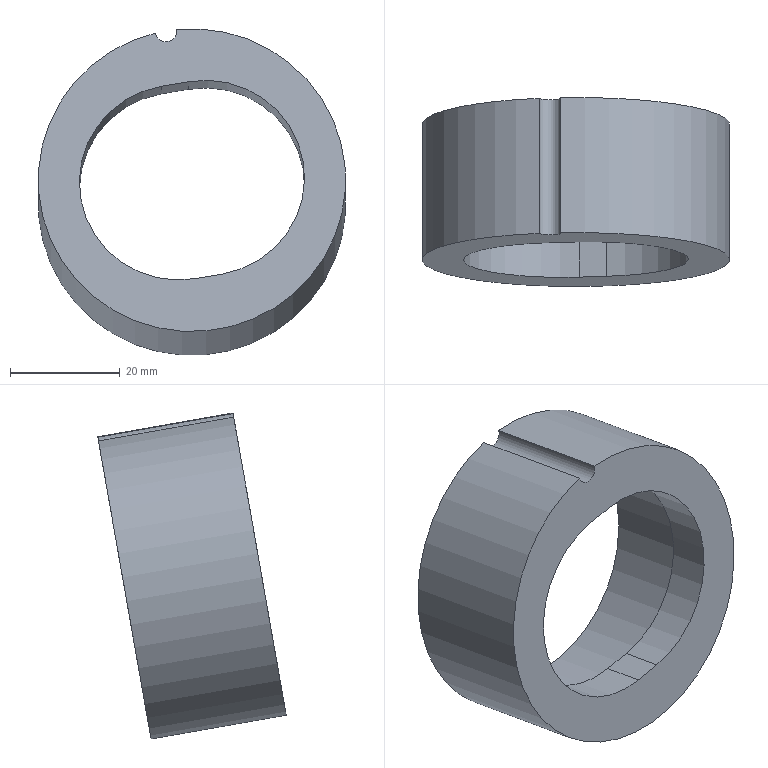Part | NX | features solid 2 | 1 solid | 10 faces | box 56 x 34.344 x 59.49 mm | volume 23536 mm3 | cylinder 5 | plane 5 | commonest cylinder face diameters 36.1 x2 4 x1 46 x1 56 x1
STEP:
#1=CARTESIAN_POINT('',(-417.763,-478.434,29.473));
#2=VERTEX_POINT('',#1);
#3=CARTESIAN_POINT('',(-417.763,-503.054,33.814));
#4=VERTEX_POINT('',#3);
#5=CARTESIAN_POINT('',(-417.763,-490.744,31.644));
#6=DIRECTION('',(0.,-0.9848,0.1736));
#7=VECTOR('',#6,1000.);
#8=LINE('',#5,#7);
#9=EDGE_CURVE('',#2,#4,#8,.T.);
#10=ORIENTED_EDGE('',*,*,#9,.T.);
#11=CARTESIAN_POINT('',(-421.702,-503.171,33.148));
#12=VERTEX_POINT('',#11);
#13=CARTESIAN_POINT('',(-415.006,-507.892,6.373));
#14=DIRECTION('',(0.,0.9848,-0.1736));
#15=DIRECTION('',(-0.1692,0.1711,0.9706));
#16=AXIS2_PLACEMENT_3D('',#13,#14,#15);
#17=CIRCLE('',#16,28.);
#18=EDGE_CURVE('',#4,#12,#17,.T.);
#19=ORIENTED_EDGE('',*,*,#18,.T.);
#20=CARTESIAN_POINT('',(-421.702,-478.551,28.807));
#21=VERTEX_POINT('',#20);
#22=CARTESIAN_POINT('',(-421.702,-490.861,30.977));
#23=DIRECTION('',(0.,-0.9848,0.1736));
#24=VECTOR('',#23,1000.);
#25=LINE('',#22,#24);
#26=EDGE_CURVE('',#12,#21,#25,.F.);
#27=ORIENTED_EDGE('',*,*,#26,.T.);
#28=CARTESIAN_POINT('',(-415.006,-483.272,2.032));
#29=DIRECTION('',(0.,0.9848,-0.1736));
#30=DIRECTION('',(-0.1692,0.1711,0.9706));
#31=AXIS2_PLACEMENT_3D('',#28,#29,#30);
#32=CIRCLE('',#31,28.);
#33=EDGE_CURVE('',#2,#21,#32,.T.);
#34=ORIENTED_EDGE('',*,*,#33,.F.);
#35=EDGE_LOOP('',(#10,#19,#27,#34));
#36=FACE_BOUND('',#35,.T.);
#37=CARTESIAN_POINT('',(-415.006,-483.272,2.032));
#38=DIRECTION('',(0.,-0.9848,0.1736));
#39=DIRECTION('',(-0.1692,0.1711,0.9706));
#40=AXIS2_PLACEMENT_3D('',#37,#38,#39);
#41=CYLINDRICAL_SURFACE('',#40,28.);
#42=ADVANCED_FACE('',(#36),#41,.T.);
#43=CARTESIAN_POINT('',(-418.898,-479.336,24.356));
#44=VERTEX_POINT('',#43);
#45=CARTESIAN_POINT('',(-415.006,-483.272,2.032));
#46=DIRECTION('',(0.,0.9848,-0.1736));
#47=DIRECTION('',(-0.1692,0.1711,0.9706));
#48=AXIS2_PLACEMENT_3D('',#45,#46,#47);
#49=CIRCLE('',#48,23.);
#50=EDGE_CURVE('',#44,#44,#49,.T.);
#51=ORIENTED_EDGE('',*,*,#50,.F.);
#52=EDGE_LOOP('',(#51));
#53=FACE_BOUND('',#52,.T.);
#54=ORIENTED_EDGE('',*,*,#33,.T.);
#55=CARTESIAN_POINT('',(-419.745,-478.48,29.209));
#56=DIRECTION('',(0.,0.9848,-0.1736));
#57=DIRECTION('',(-0.1692,0.1711,0.9706));
#58=AXIS2_PLACEMENT_3D('',#55,#56,#57);
#59=CIRCLE('',#58,2.);
#60=EDGE_CURVE('',#2,#21,#59,.T.);
#61=ORIENTED_EDGE('',*,*,#60,.F.);
#62=EDGE_LOOP('',(#54,#61));
#63=FACE_BOUND('',#62,.T.);
#64=CARTESIAN_POINT('',(-415.006,-483.272,2.032));
#65=DIRECTION('',(0.,-0.9848,0.1736));
#66=DIRECTION('',(-0.1692,0.1711,0.9706));
#67=AXIS2_PLACEMENT_3D('',#64,#65,#66);
#68=PLANE('',#67);
#69=ADVANCED_FACE('',(#53,#63),#68,.F.);
#70=CARTESIAN_POINT('',(-409.488,-510.908,-10.729));
#71=VERTEX_POINT('',#70);
#72=CARTESIAN_POINT('',(-414.415,-511.055,-11.563));
#73=VERTEX_POINT('',#72);
#74=CARTESIAN_POINT('',(-409.488,-510.908,-10.729));
#75=DIRECTION('',(-0.9856,-0.02939,-0.1667));
#76=VECTOR('',#75,1000.);
#77=LINE('',#74,#76);
#78=EDGE_CURVE('',#71,#73,#77,.T.);
#79=ORIENTED_EDGE('',*,*,#78,.T.);
#80=CARTESIAN_POINT('',(-420.525,-504.877,23.476));
#81=VERTEX_POINT('',#80);
#82=CARTESIAN_POINT('',(-417.47,-507.966,5.957));
#83=DIRECTION('',(0.,0.9848,-0.1736));
#84=DIRECTION('',(-0.1692,0.1711,0.9706));
#85=AXIS2_PLACEMENT_3D('',#82,#83,#84);
#86=CIRCLE('',#85,18.05);
#87=EDGE_CURVE('',#73,#81,#86,.T.);
#88=ORIENTED_EDGE('',*,*,#87,.T.);
#89=CARTESIAN_POINT('',(-415.597,-504.73,24.31));
#90=VERTEX_POINT('',#89);
#91=CARTESIAN_POINT('',(-415.597,-504.73,24.31));
#92=DIRECTION('',(-0.9856,-0.02939,-0.1667));
#93=VECTOR('',#92,1000.);
#94=LINE('',#91,#93);
#95=EDGE_CURVE('',#90,#81,#94,.T.);
#96=ORIENTED_EDGE('',*,*,#95,.F.);
#97=CARTESIAN_POINT('',(-412.542,-507.819,6.79));
#98=DIRECTION('',(0.,0.9848,-0.1736));
#99=DIRECTION('',(-0.1692,0.1711,0.9706));
#100=AXIS2_PLACEMENT_3D('',#97,#98,#99);
#101=CIRCLE('',#100,18.05);
#102=EDGE_CURVE('',#90,#71,#101,.T.);
#103=ORIENTED_EDGE('',*,*,#102,.T.);
#104=EDGE_LOOP('',(#79,#88,#96,#103));
#105=FACE_BOUND('',#104,.T.);
#106=CARTESIAN_POINT('',(-419.745,-503.1,33.55));
#107=DIRECTION('',(0.,0.9848,-0.1736));
#108=DIRECTION('',(-0.1692,0.1711,0.9706));
#109=AXIS2_PLACEMENT_3D('',#106,#107,#108);
#110=CIRCLE('',#109,2.);
#111=EDGE_CURVE('',#4,#12,#110,.T.);
#112=ORIENTED_EDGE('',*,*,#111,.T.);
#113=ORIENTED_EDGE('',*,*,#18,.F.);
#114=EDGE_LOOP('',(#112,#113));
#115=FACE_BOUND('',#114,.T.);
#116=CARTESIAN_POINT('',(-415.006,-507.892,6.373));
#117=DIRECTION('',(0.,-0.9848,0.1736));
#118=DIRECTION('',(-0.1692,0.1711,0.9706));
#119=AXIS2_PLACEMENT_3D('',#116,#117,#118);
#120=PLANE('',#119);
#121=ADVANCED_FACE('',(#105,#115),#120,.T.);
#122=ORIENTED_EDGE('',*,*,#50,.T.);
#123=EDGE_LOOP('',(#122));
#124=FACE_BOUND('',#123,.T.);
#125=CARTESIAN_POINT('',(-418.898,-496.078,27.308));
#126=VERTEX_POINT('',#125);
#127=CARTESIAN_POINT('',(-415.006,-500.014,4.984));
#128=DIRECTION('',(0.,0.9848,-0.1736));
#129=DIRECTION('',(-0.1692,0.1711,0.9706));
#130=AXIS2_PLACEMENT_3D('',#127,#128,#129);
#131=CIRCLE('',#130,23.);
#132=EDGE_CURVE('',#126,#126,#131,.T.);
#133=ORIENTED_EDGE('',*,*,#132,.F.);
#134=EDGE_LOOP('',(#133));
#135=FACE_BOUND('',#134,.T.);
#136=CARTESIAN_POINT('',(-415.006,-483.272,2.032));
#137=DIRECTION('',(0.,-0.9848,0.1736));
#138=DIRECTION('',(-0.1692,0.1711,0.9706));
#139=AXIS2_PLACEMENT_3D('',#136,#137,#138);
#140=CYLINDRICAL_SURFACE('',#139,23.);
#141=ADVANCED_FACE('',(#124,#135),#140,.F.);
#142=CARTESIAN_POINT('',(-415.597,-496.851,22.92));
#143=VERTEX_POINT('',#142);
#144=CARTESIAN_POINT('',(-409.488,-503.03,-12.118));
#145=VERTEX_POINT('',#144);
#146=CARTESIAN_POINT('',(-412.542,-499.941,5.401));
#147=DIRECTION('',(0.,0.9848,-0.1736));
#148=DIRECTION('',(-0.1692,0.1711,0.9706));
#149=AXIS2_PLACEMENT_3D('',#146,#147,#148);
#150=CIRCLE('',#149,18.05);
#151=EDGE_CURVE('',#143,#145,#150,.T.);
#152=ORIENTED_EDGE('',*,*,#151,.F.);
#153=CARTESIAN_POINT('',(-420.525,-496.998,22.087));
#154=VERTEX_POINT('',#153);
#155=CARTESIAN_POINT('',(-418.061,-496.925,22.504));
#156=DIRECTION('',(-0.9856,-0.02939,-0.1667));
#157=VECTOR('',#156,1000.);
#158=LINE('',#155,#157);
#159=EDGE_CURVE('',#143,#154,#158,.T.);
#160=ORIENTED_EDGE('',*,*,#159,.T.);
#161=CARTESIAN_POINT('',(-414.415,-503.177,-12.952));
#162=VERTEX_POINT('',#161);
#163=CARTESIAN_POINT('',(-417.47,-500.087,4.568));
#164=DIRECTION('',(0.,0.9848,-0.1736));
#165=DIRECTION('',(-0.1692,0.1711,0.9706));
#166=AXIS2_PLACEMENT_3D('',#163,#164,#165);
#167=CIRCLE('',#166,18.05);
#168=EDGE_CURVE('',#162,#154,#167,.T.);
#169=ORIENTED_EDGE('',*,*,#168,.F.);
#170=CARTESIAN_POINT('',(-411.952,-503.103,-12.535));
#171=DIRECTION('',(-0.9856,-0.02939,-0.1667));
#172=VECTOR('',#171,1000.);
#173=LINE('',#170,#172);
#174=EDGE_CURVE('',#145,#162,#173,.T.);
#175=ORIENTED_EDGE('',*,*,#174,.F.);
#176=EDGE_LOOP('',(#152,#160,#169,#175));
#177=FACE_BOUND('',#176,.T.);
#178=ORIENTED_EDGE('',*,*,#132,.T.);
#179=EDGE_LOOP('',(#178));
#180=FACE_BOUND('',#179,.T.);
#181=CARTESIAN_POINT('',(-415.006,-500.014,4.984));
#182=DIRECTION('',(0.,-0.9848,0.1736));
#183=DIRECTION('',(-0.1692,0.1711,0.9706));
#184=AXIS2_PLACEMENT_3D('',#181,#182,#183);
#185=PLANE('',#184);
#186=ADVANCED_FACE('',(#177,#180),#185,.F.);
#187=ORIENTED_EDGE('',*,*,#9,.F.);
#188=ORIENTED_EDGE('',*,*,#60,.T.);
#189=ORIENTED_EDGE('',*,*,#26,.F.);
#190=ORIENTED_EDGE('',*,*,#111,.F.);
#191=EDGE_LOOP('',(#187,#188,#189,#190));
#192=FACE_BOUND('',#191,.T.);
#193=CARTESIAN_POINT('',(-419.745,-478.48,29.209));
#194=DIRECTION('',(0.,-0.9848,0.1736));
#195=DIRECTION('',(-0.1692,0.1711,0.9706));
#196=AXIS2_PLACEMENT_3D('',#193,#194,#195);
#197=CYLINDRICAL_SURFACE('',#196,2.);
#198=ADVANCED_FACE('',(#192),#197,.F.);
#199=CARTESIAN_POINT('',(-409.488,-486.288,-15.07));
#200=DIRECTION('',(0.,-0.9848,0.1736));
#201=VECTOR('',#200,1000.);
#202=LINE('',#199,#201);
#203=EDGE_CURVE('',#145,#71,#202,.T.);
#204=ORIENTED_EDGE('',*,*,#203,.F.);
#205=ORIENTED_EDGE('',*,*,#174,.T.);
#206=CARTESIAN_POINT('',(-414.415,-486.435,-15.904));
#207=DIRECTION('',(0.,-0.9848,0.1736));
#208=VECTOR('',#207,1000.);
#209=LINE('',#206,#208);
#210=EDGE_CURVE('',#162,#73,#209,.T.);
#211=ORIENTED_EDGE('',*,*,#210,.T.);
#212=ORIENTED_EDGE('',*,*,#78,.F.);
#213=EDGE_LOOP('',(#204,#205,#211,#212));
#214=FACE_BOUND('',#213,.T.);
#215=CARTESIAN_POINT('',(-409.488,-486.288,-15.07));
#216=DIRECTION('',(0.1692,-0.1711,-0.9706));
#217=DIRECTION('',(0.,-0.9848,0.1736));
#218=AXIS2_PLACEMENT_3D('',#215,#216,#217);
#219=PLANE('',#218);
#220=ADVANCED_FACE('',(#214),#219,.F.);
#221=ORIENTED_EDGE('',*,*,#210,.F.);
#222=ORIENTED_EDGE('',*,*,#168,.T.);
#223=CARTESIAN_POINT('',(-420.525,-480.257,19.135));
#224=DIRECTION('',(0.,-0.9848,0.1736));
#225=VECTOR('',#224,1000.);
#226=LINE('',#223,#225);
#227=EDGE_CURVE('',#154,#81,#226,.T.);
#228=ORIENTED_EDGE('',*,*,#227,.T.);
#229=ORIENTED_EDGE('',*,*,#87,.F.);
#230=EDGE_LOOP('',(#221,#222,#228,#229));
#231=FACE_BOUND('',#230,.T.);
#232=CARTESIAN_POINT('',(-417.47,-483.346,1.616));
#233=DIRECTION('',(0.,-0.9848,0.1736));
#234=DIRECTION('',(-0.1692,0.1711,0.9706));
#235=AXIS2_PLACEMENT_3D('',#232,#233,#234);
#236=CYLINDRICAL_SURFACE('',#235,18.05);
#237=ADVANCED_FACE('',(#231),#236,.F.);
#238=ORIENTED_EDGE('',*,*,#159,.F.);
#239=CARTESIAN_POINT('',(-415.597,-480.11,19.968));
#240=DIRECTION('',(0.,-0.9848,0.1736));
#241=VECTOR('',#240,1000.);
#242=LINE('',#239,#241);
#243=EDGE_CURVE('',#143,#90,#242,.T.);
#244=ORIENTED_EDGE('',*,*,#243,.T.);
#245=ORIENTED_EDGE('',*,*,#95,.T.);
#246=ORIENTED_EDGE('',*,*,#227,.F.);
#247=EDGE_LOOP('',(#238,#244,#245,#246));
#248=FACE_BOUND('',#247,.T.);
#249=CARTESIAN_POINT('',(-415.597,-480.11,19.968));
#250=DIRECTION('',(0.1692,-0.1711,-0.9706));
#251=DIRECTION('',(0.,-0.9848,0.1736));
#252=AXIS2_PLACEMENT_3D('',#249,#250,#251);
#253=PLANE('',#252);
#254=ADVANCED_FACE('',(#248),#253,.T.);
#255=ORIENTED_EDGE('',*,*,#243,.F.);
#256=ORIENTED_EDGE('',*,*,#151,.T.);
#257=ORIENTED_EDGE('',*,*,#203,.T.);
#258=ORIENTED_EDGE('',*,*,#102,.F.);
#259=EDGE_LOOP('',(#255,#256,#257,#258));
#260=FACE_BOUND('',#259,.T.);
#261=CARTESIAN_POINT('',(-412.542,-483.199,2.449));
#262=DIRECTION('',(0.,-0.9848,0.1736));
#263=DIRECTION('',(-0.1692,0.1711,0.9706));
#264=AXIS2_PLACEMENT_3D('',#261,#262,#263);
#265=CYLINDRICAL_SURFACE('',#264,18.05);
#266=ADVANCED_FACE('',(#260),#265,.F.);
#267=CLOSED_SHELL('',(#42,#69,#121,#141,#186,#198,#220,#237,#254,#266));
#268=MANIFOLD_SOLID_BREP('',#267);
#269=(LENGTH_UNIT()NAMED_UNIT(*)SI_UNIT(.MILLI.,.METRE.));
#270=UNCERTAINTY_MEASURE_WITH_UNIT(LENGTH_MEASURE(0.00001),#269,'','');
#271=(NAMED_UNIT(*)PLANE_ANGLE_UNIT()SI_UNIT($,.RADIAN.));
#272=(NAMED_UNIT(*)SI_UNIT($,.STERADIAN.)SOLID_ANGLE_UNIT());
#273=(GEOMETRIC_REPRESENTATION_CONTEXT(3)GLOBAL_UNCERTAINTY_ASSIGNED_CONTEXT((#270))GLOBAL_UNIT_ASSIGNED_CONTEXT((#269,#271,#272))REPRESENTATION_CONTEXT('',''));
#274=ADVANCED_BREP_SHAPE_REPRESENTATION('',(#268),#273);